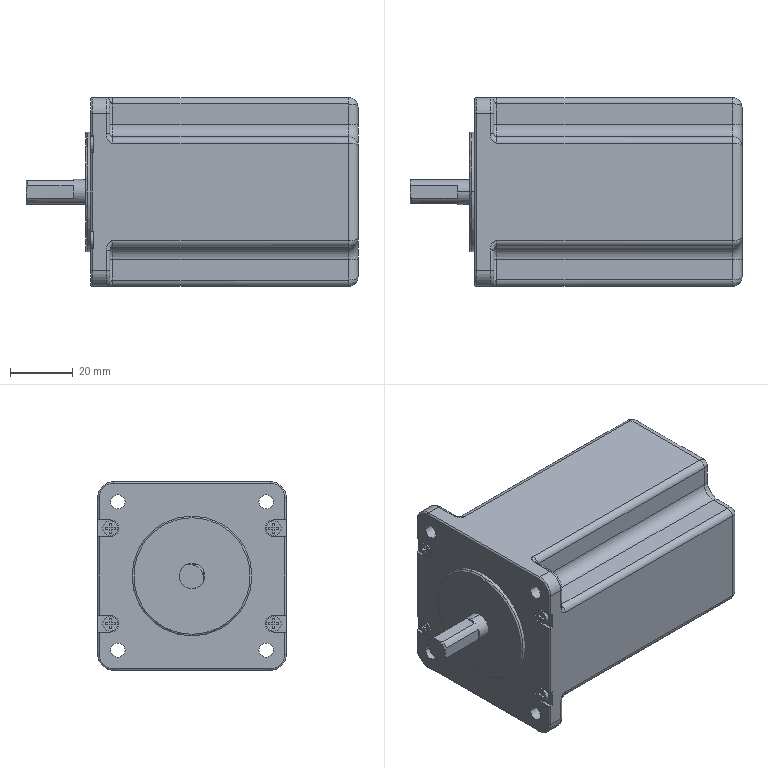Part | STEP file | Stepper motor SS2403A42A | 1 solid | 203 faces | box 105.6 x 60 x 60 mm | volume 258866 mm3 | plane 92 | cylinder 76 | torus 18 | spline 16 | cone 1 | commonest cylinder face diameters 2 x16 6 x12 1 x8 4 x8 4.52 x8 4.739 x8